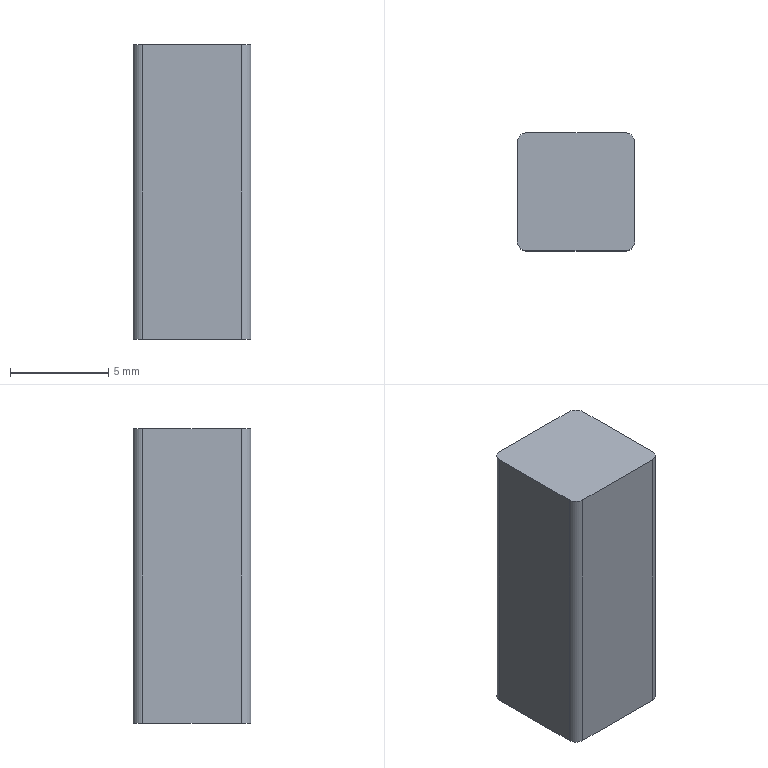Part | NX | features BREP 1 | 1 solid | 10 faces | box 6 x 6 x 15 mm | volume 536.781 mm3 | plane 6 | cylinder 4 | commonest cylinder face diameters 1 x4
STEP:
#1=CARTESIAN_POINT('',(-2.5,3.,-25.6));
#2=VERTEX_POINT('',#1);
#3=CARTESIAN_POINT('',(-3.,2.5,-25.6));
#4=VERTEX_POINT('',#3);
#5=CARTESIAN_POINT('',(-2.5,2.5,-25.6));
#6=DIRECTION('',(0.,0.,1.));
#7=DIRECTION('',(1.,0.,0.));
#8=AXIS2_PLACEMENT_3D('',#5,#6,#7);
#9=CIRCLE('',#8,0.5);
#10=EDGE_CURVE('',#2,#4,#9,.T.);
#11=ORIENTED_EDGE('',*,*,#10,.F.);
#12=CARTESIAN_POINT('',(-2.5,3.,-40.6));
#13=VERTEX_POINT('',#12);
#14=CARTESIAN_POINT('',(-2.5,3.,-40.6));
#15=DIRECTION('',(0.,0.,1.));
#16=VECTOR('',#15,1000.);
#17=LINE('',#14,#16);
#18=EDGE_CURVE('',#13,#2,#17,.T.);
#19=ORIENTED_EDGE('',*,*,#18,.F.);
#20=CARTESIAN_POINT('',(-3.,2.5,-40.6));
#21=VERTEX_POINT('',#20);
#22=CARTESIAN_POINT('',(-2.5,2.5,-40.6));
#23=DIRECTION('',(0.,0.,1.));
#24=DIRECTION('',(1.,0.,0.));
#25=AXIS2_PLACEMENT_3D('',#22,#23,#24);
#26=CIRCLE('',#25,0.5);
#27=EDGE_CURVE('',#13,#21,#26,.T.);
#28=ORIENTED_EDGE('',*,*,#27,.T.);
#29=CARTESIAN_POINT('',(-3.,2.5,-40.6));
#30=DIRECTION('',(0.,0.,1.));
#31=VECTOR('',#30,1000.);
#32=LINE('',#29,#31);
#33=EDGE_CURVE('',#21,#4,#32,.T.);
#34=ORIENTED_EDGE('',*,*,#33,.T.);
#35=EDGE_LOOP('',(#11,#19,#28,#34));
#36=FACE_BOUND('',#35,.T.);
#37=CARTESIAN_POINT('',(-2.5,2.5,-40.6));
#38=DIRECTION('',(0.,0.,1.));
#39=DIRECTION('',(-1.,0.,0.));
#40=AXIS2_PLACEMENT_3D('',#37,#38,#39);
#41=CYLINDRICAL_SURFACE('',#40,0.5);
#42=ADVANCED_FACE('',(#36),#41,.T.);
#43=CARTESIAN_POINT('',(-3.,-2.5,-25.6));
#44=VERTEX_POINT('',#43);
#45=CARTESIAN_POINT('',(-3.,-2.5,-25.6));
#46=DIRECTION('',(0.,1.,0.));
#47=VECTOR('',#46,1000.);
#48=LINE('',#45,#47);
#49=EDGE_CURVE('',#44,#4,#48,.T.);
#50=ORIENTED_EDGE('',*,*,#49,.T.);
#51=ORIENTED_EDGE('',*,*,#33,.F.);
#52=CARTESIAN_POINT('',(-3.,-2.5,-40.6));
#53=VERTEX_POINT('',#52);
#54=CARTESIAN_POINT('',(-3.,-2.5,-40.6));
#55=DIRECTION('',(0.,1.,0.));
#56=VECTOR('',#55,1000.);
#57=LINE('',#54,#56);
#58=EDGE_CURVE('',#53,#21,#57,.T.);
#59=ORIENTED_EDGE('',*,*,#58,.F.);
#60=CARTESIAN_POINT('',(-3.,-2.5,-40.6));
#61=DIRECTION('',(0.,0.,1.));
#62=VECTOR('',#61,1000.);
#63=LINE('',#60,#62);
#64=EDGE_CURVE('',#53,#44,#63,.T.);
#65=ORIENTED_EDGE('',*,*,#64,.T.);
#66=EDGE_LOOP('',(#50,#51,#59,#65));
#67=FACE_BOUND('',#66,.T.);
#68=CARTESIAN_POINT('',(-3.,-2.5,-40.6));
#69=DIRECTION('',(1.,0.,0.));
#70=DIRECTION('',(0.,0.,1.));
#71=AXIS2_PLACEMENT_3D('',#68,#69,#70);
#72=PLANE('',#71);
#73=ADVANCED_FACE('',(#67),#72,.F.);
#74=CARTESIAN_POINT('',(-2.5,-3.,-25.6));
#75=VERTEX_POINT('',#74);
#76=CARTESIAN_POINT('',(-2.5,-2.5,-25.6));
#77=DIRECTION('',(0.,0.,1.));
#78=DIRECTION('',(1.,0.,0.));
#79=AXIS2_PLACEMENT_3D('',#76,#77,#78);
#80=CIRCLE('',#79,0.5);
#81=EDGE_CURVE('',#44,#75,#80,.T.);
#82=ORIENTED_EDGE('',*,*,#81,.F.);
#83=ORIENTED_EDGE('',*,*,#64,.F.);
#84=CARTESIAN_POINT('',(-2.5,-3.,-40.6));
#85=VERTEX_POINT('',#84);
#86=CARTESIAN_POINT('',(-2.5,-2.5,-40.6));
#87=DIRECTION('',(0.,0.,1.));
#88=DIRECTION('',(1.,0.,0.));
#89=AXIS2_PLACEMENT_3D('',#86,#87,#88);
#90=CIRCLE('',#89,0.5);
#91=EDGE_CURVE('',#53,#85,#90,.T.);
#92=ORIENTED_EDGE('',*,*,#91,.T.);
#93=CARTESIAN_POINT('',(-2.5,-3.,-40.6));
#94=DIRECTION('',(0.,0.,1.));
#95=VECTOR('',#94,1000.);
#96=LINE('',#93,#95);
#97=EDGE_CURVE('',#85,#75,#96,.T.);
#98=ORIENTED_EDGE('',*,*,#97,.T.);
#99=EDGE_LOOP('',(#82,#83,#92,#98));
#100=FACE_BOUND('',#99,.T.);
#101=CARTESIAN_POINT('',(-2.5,-2.5,-40.6));
#102=DIRECTION('',(0.,0.,1.));
#103=DIRECTION('',(-1.,0.,0.));
#104=AXIS2_PLACEMENT_3D('',#101,#102,#103);
#105=CYLINDRICAL_SURFACE('',#104,0.5);
#106=ADVANCED_FACE('',(#100),#105,.T.);
#107=CARTESIAN_POINT('',(2.5,-3.,-25.6));
#108=VERTEX_POINT('',#107);
#109=CARTESIAN_POINT('',(2.5,-3.,-25.6));
#110=DIRECTION('',(-1.,0.,0.));
#111=VECTOR('',#110,1000.);
#112=LINE('',#109,#111);
#113=EDGE_CURVE('',#108,#75,#112,.T.);
#114=ORIENTED_EDGE('',*,*,#113,.T.);
#115=ORIENTED_EDGE('',*,*,#97,.F.);
#116=CARTESIAN_POINT('',(2.5,-3.,-40.6));
#117=VERTEX_POINT('',#116);
#118=CARTESIAN_POINT('',(2.5,-3.,-40.6));
#119=DIRECTION('',(-1.,0.,0.));
#120=VECTOR('',#119,1000.);
#121=LINE('',#118,#120);
#122=EDGE_CURVE('',#117,#85,#121,.T.);
#123=ORIENTED_EDGE('',*,*,#122,.F.);
#124=CARTESIAN_POINT('',(2.5,-3.,-40.6));
#125=DIRECTION('',(0.,0.,1.));
#126=VECTOR('',#125,1000.);
#127=LINE('',#124,#126);
#128=EDGE_CURVE('',#117,#108,#127,.T.);
#129=ORIENTED_EDGE('',*,*,#128,.T.);
#130=EDGE_LOOP('',(#114,#115,#123,#129));
#131=FACE_BOUND('',#130,.T.);
#132=CARTESIAN_POINT('',(2.5,-3.,-40.6));
#133=DIRECTION('',(0.,1.,0.));
#134=DIRECTION('',(0.,0.,-1.));
#135=AXIS2_PLACEMENT_3D('',#132,#133,#134);
#136=PLANE('',#135);
#137=ADVANCED_FACE('',(#131),#136,.F.);
#138=CARTESIAN_POINT('',(3.,-2.5,-25.6));
#139=VERTEX_POINT('',#138);
#140=CARTESIAN_POINT('',(2.5,-2.5,-25.6));
#141=DIRECTION('',(0.,0.,1.));
#142=DIRECTION('',(1.,0.,0.));
#143=AXIS2_PLACEMENT_3D('',#140,#141,#142);
#144=CIRCLE('',#143,0.5);
#145=EDGE_CURVE('',#108,#139,#144,.T.);
#146=ORIENTED_EDGE('',*,*,#145,.F.);
#147=ORIENTED_EDGE('',*,*,#128,.F.);
#148=CARTESIAN_POINT('',(3.,-2.5,-40.6));
#149=VERTEX_POINT('',#148);
#150=CARTESIAN_POINT('',(2.5,-2.5,-40.6));
#151=DIRECTION('',(0.,0.,1.));
#152=DIRECTION('',(1.,0.,0.));
#153=AXIS2_PLACEMENT_3D('',#150,#151,#152);
#154=CIRCLE('',#153,0.5);
#155=EDGE_CURVE('',#117,#149,#154,.T.);
#156=ORIENTED_EDGE('',*,*,#155,.T.);
#157=CARTESIAN_POINT('',(3.,-2.5,-40.6));
#158=DIRECTION('',(0.,0.,1.));
#159=VECTOR('',#158,1000.);
#160=LINE('',#157,#159);
#161=EDGE_CURVE('',#149,#139,#160,.T.);
#162=ORIENTED_EDGE('',*,*,#161,.T.);
#163=EDGE_LOOP('',(#146,#147,#156,#162));
#164=FACE_BOUND('',#163,.T.);
#165=CARTESIAN_POINT('',(2.5,-2.5,-40.6));
#166=DIRECTION('',(0.,0.,1.));
#167=DIRECTION('',(-1.,0.,0.));
#168=AXIS2_PLACEMENT_3D('',#165,#166,#167);
#169=CYLINDRICAL_SURFACE('',#168,0.5);
#170=ADVANCED_FACE('',(#164),#169,.T.);
#171=CARTESIAN_POINT('',(3.,2.5,-25.6));
#172=VERTEX_POINT('',#171);
#173=CARTESIAN_POINT('',(3.,2.5,-25.6));
#174=DIRECTION('',(0.,-1.,0.));
#175=VECTOR('',#174,1000.);
#176=LINE('',#173,#175);
#177=EDGE_CURVE('',#172,#139,#176,.T.);
#178=ORIENTED_EDGE('',*,*,#177,.T.);
#179=ORIENTED_EDGE('',*,*,#161,.F.);
#180=CARTESIAN_POINT('',(3.,2.5,-40.6));
#181=VERTEX_POINT('',#180);
#182=CARTESIAN_POINT('',(3.,2.5,-40.6));
#183=DIRECTION('',(0.,-1.,0.));
#184=VECTOR('',#183,1000.);
#185=LINE('',#182,#184);
#186=EDGE_CURVE('',#181,#149,#185,.T.);
#187=ORIENTED_EDGE('',*,*,#186,.F.);
#188=CARTESIAN_POINT('',(3.,2.5,-40.6));
#189=DIRECTION('',(0.,0.,1.));
#190=VECTOR('',#189,1000.);
#191=LINE('',#188,#190);
#192=EDGE_CURVE('',#181,#172,#191,.T.);
#193=ORIENTED_EDGE('',*,*,#192,.T.);
#194=EDGE_LOOP('',(#178,#179,#187,#193));
#195=FACE_BOUND('',#194,.T.);
#196=CARTESIAN_POINT('',(3.,2.5,-40.6));
#197=DIRECTION('',(-1.,0.,0.));
#198=DIRECTION('',(0.,0.,-1.));
#199=AXIS2_PLACEMENT_3D('',#196,#197,#198);
#200=PLANE('',#199);
#201=ADVANCED_FACE('',(#195),#200,.F.);
#202=CARTESIAN_POINT('',(2.5,3.,-25.6));
#203=VERTEX_POINT('',#202);
#204=CARTESIAN_POINT('',(2.5,2.5,-25.6));
#205=DIRECTION('',(0.,0.,1.));
#206=DIRECTION('',(1.,0.,0.));
#207=AXIS2_PLACEMENT_3D('',#204,#205,#206);
#208=CIRCLE('',#207,0.5);
#209=EDGE_CURVE('',#172,#203,#208,.T.);
#210=ORIENTED_EDGE('',*,*,#209,.F.);
#211=ORIENTED_EDGE('',*,*,#192,.F.);
#212=CARTESIAN_POINT('',(2.5,3.,-40.6));
#213=VERTEX_POINT('',#212);
#214=CARTESIAN_POINT('',(2.5,2.5,-40.6));
#215=DIRECTION('',(0.,0.,1.));
#216=DIRECTION('',(1.,0.,0.));
#217=AXIS2_PLACEMENT_3D('',#214,#215,#216);
#218=CIRCLE('',#217,0.5);
#219=EDGE_CURVE('',#181,#213,#218,.T.);
#220=ORIENTED_EDGE('',*,*,#219,.T.);
#221=CARTESIAN_POINT('',(2.5,3.,-40.6));
#222=DIRECTION('',(0.,0.,1.));
#223=VECTOR('',#222,1000.);
#224=LINE('',#221,#223);
#225=EDGE_CURVE('',#213,#203,#224,.T.);
#226=ORIENTED_EDGE('',*,*,#225,.T.);
#227=EDGE_LOOP('',(#210,#211,#220,#226));
#228=FACE_BOUND('',#227,.T.);
#229=CARTESIAN_POINT('',(2.5,2.5,-40.6));
#230=DIRECTION('',(0.,0.,1.));
#231=DIRECTION('',(-1.,0.,0.));
#232=AXIS2_PLACEMENT_3D('',#229,#230,#231);
#233=CYLINDRICAL_SURFACE('',#232,0.5);
#234=ADVANCED_FACE('',(#228),#233,.T.);
#235=CARTESIAN_POINT('',(-2.5,3.,-25.6));
#236=DIRECTION('',(1.,0.,0.));
#237=VECTOR('',#236,1000.);
#238=LINE('',#235,#237);
#239=EDGE_CURVE('',#2,#203,#238,.T.);
#240=ORIENTED_EDGE('',*,*,#239,.T.);
#241=ORIENTED_EDGE('',*,*,#225,.F.);
#242=CARTESIAN_POINT('',(-2.5,3.,-40.6));
#243=DIRECTION('',(1.,0.,0.));
#244=VECTOR('',#243,1000.);
#245=LINE('',#242,#244);
#246=EDGE_CURVE('',#13,#213,#245,.T.);
#247=ORIENTED_EDGE('',*,*,#246,.F.);
#248=ORIENTED_EDGE('',*,*,#18,.T.);
#249=EDGE_LOOP('',(#240,#241,#247,#248));
#250=FACE_BOUND('',#249,.T.);
#251=CARTESIAN_POINT('',(-2.5,3.,-40.6));
#252=DIRECTION('',(0.,-1.,0.));
#253=DIRECTION('',(0.,0.,1.));
#254=AXIS2_PLACEMENT_3D('',#251,#252,#253);
#255=PLANE('',#254);
#256=ADVANCED_FACE('',(#250),#255,.F.);
#257=ORIENTED_EDGE('',*,*,#27,.F.);
#258=ORIENTED_EDGE('',*,*,#246,.T.);
#259=ORIENTED_EDGE('',*,*,#219,.F.);
#260=ORIENTED_EDGE('',*,*,#186,.T.);
#261=ORIENTED_EDGE('',*,*,#155,.F.);
#262=ORIENTED_EDGE('',*,*,#122,.T.);
#263=ORIENTED_EDGE('',*,*,#91,.F.);
#264=ORIENTED_EDGE('',*,*,#58,.T.);
#265=EDGE_LOOP('',(#257,#258,#259,#260,#261,#262,#263,#264));
#266=FACE_BOUND('',#265,.T.);
#267=CARTESIAN_POINT('',(-2.5,2.5,-40.6));
#268=DIRECTION('',(0.,0.,1.));
#269=DIRECTION('',(-1.,0.,0.));
#270=AXIS2_PLACEMENT_3D('',#267,#268,#269);
#271=PLANE('',#270);
#272=ADVANCED_FACE('',(#266),#271,.F.);
#273=ORIENTED_EDGE('',*,*,#10,.T.);
#274=ORIENTED_EDGE('',*,*,#49,.F.);
#275=ORIENTED_EDGE('',*,*,#81,.T.);
#276=ORIENTED_EDGE('',*,*,#113,.F.);
#277=ORIENTED_EDGE('',*,*,#145,.T.);
#278=ORIENTED_EDGE('',*,*,#177,.F.);
#279=ORIENTED_EDGE('',*,*,#209,.T.);
#280=ORIENTED_EDGE('',*,*,#239,.F.);
#281=EDGE_LOOP('',(#273,#274,#275,#276,#277,#278,#279,#280));
#282=FACE_BOUND('',#281,.T.);
#283=CARTESIAN_POINT('',(-2.5,2.5,-25.6));
#284=DIRECTION('',(0.,0.,1.));
#285=DIRECTION('',(-1.,0.,0.));
#286=AXIS2_PLACEMENT_3D('',#283,#284,#285);
#287=PLANE('',#286);
#288=ADVANCED_FACE('',(#282),#287,.T.);
#289=CLOSED_SHELL('',(#42,#73,#106,#137,#170,#201,#234,#256,#272,#288));
#290=MANIFOLD_SOLID_BREP('',#289);
#291=(LENGTH_UNIT()NAMED_UNIT(*)SI_UNIT(.MILLI.,.METRE.));
#292=UNCERTAINTY_MEASURE_WITH_UNIT(LENGTH_MEASURE(0.00001),#291,'','');
#293=(NAMED_UNIT(*)PLANE_ANGLE_UNIT()SI_UNIT($,.RADIAN.));
#294=(NAMED_UNIT(*)SI_UNIT($,.STERADIAN.)SOLID_ANGLE_UNIT());
#295=(GEOMETRIC_REPRESENTATION_CONTEXT(3)GLOBAL_UNCERTAINTY_ASSIGNED_CONTEXT((#292))GLOBAL_UNIT_ASSIGNED_CONTEXT((#291,#293,#294))REPRESENTATION_CONTEXT('',''));
#296=ADVANCED_BREP_SHAPE_REPRESENTATION('',(#290),#295);